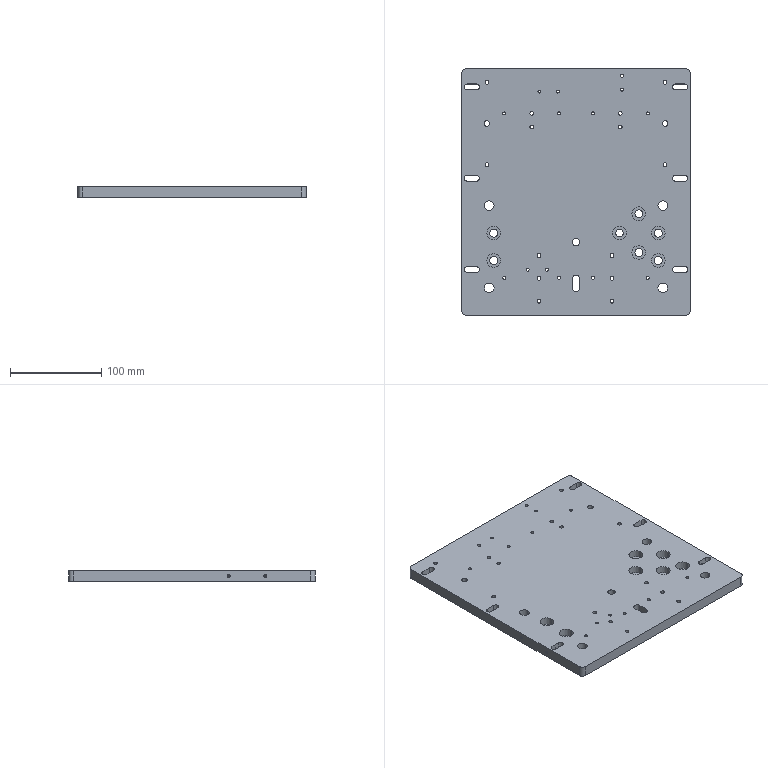Part | STEP file | 03-26压机底Plate | 1 solid | 177 faces | box 250 x 270 x 12 mm | volume 774847 mm3 | cylinder 138 | plane 31 | cone 8 | commonest cylinder face diameters 3.3 x36 4.2 x20 6.5 x18 15 x14 4 x8 9 x8